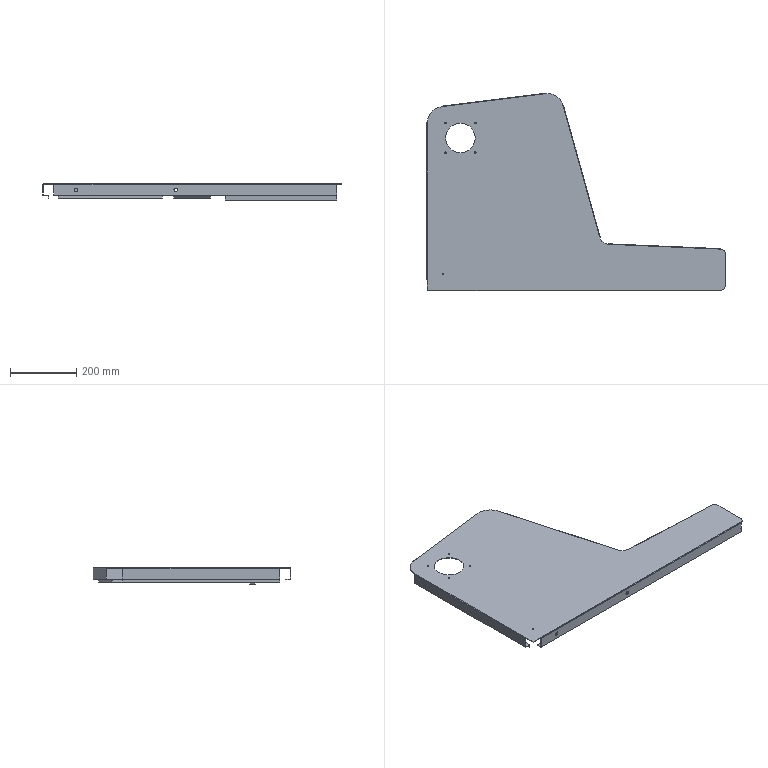Part | SolidWorks | features EdgeFlange 15, ICE 4, FlatPattern 1, SMBaseFlange 1, SheetMetal 1 | 1 solid | 132 faces | box 898.5 x 594.649 x 48.5 mm | volume 675407 mm3 | plane 95 | cylinder 37 | commonest cylinder face diameters 3 x14 5 x8 10 x4 2.5 x2 4.5 x2 27 x2